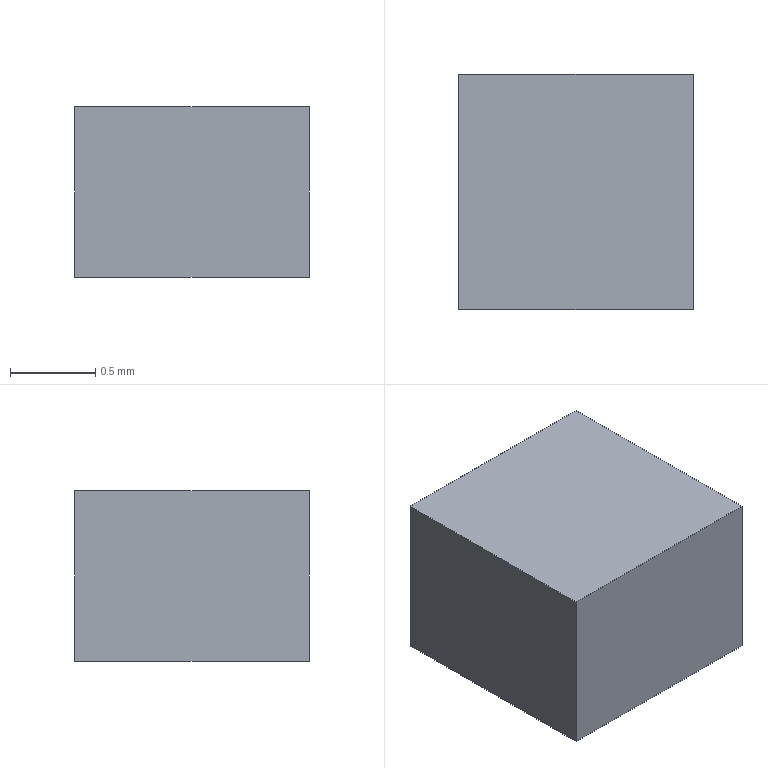Part | SolidWorks | features BaseBody 1 | 1 solid | 6 faces | box 1.375 x 1.375 x 1 mm | volume 1.891 mm3 | plane 6
STEP:
#1=CARTESIAN_POINT('',(7.625,9.125,1.5));
#2=VERTEX_POINT('',#1);
#3=CARTESIAN_POINT('',(7.625,7.75,1.5));
#4=VERTEX_POINT('',#3);
#5=CARTESIAN_POINT('',(7.625,9.125,1.5));
#6=DIRECTION('',(0.,-1.,0.));
#7=VECTOR('',#6,1000.);
#8=LINE('',#5,#7);
#9=EDGE_CURVE('',#2,#4,#8,.T.);
#10=ORIENTED_EDGE('',*,*,#9,.T.);
#11=CARTESIAN_POINT('',(7.625,7.75,2.5));
#12=VERTEX_POINT('',#11);
#13=CARTESIAN_POINT('',(7.625,7.75,2.5));
#14=DIRECTION('',(0.,0.,-1.));
#15=VECTOR('',#14,1000.);
#16=LINE('',#13,#15);
#17=EDGE_CURVE('',#12,#4,#16,.T.);
#18=ORIENTED_EDGE('',*,*,#17,.F.);
#19=CARTESIAN_POINT('',(7.625,9.125,2.5));
#20=VERTEX_POINT('',#19);
#21=CARTESIAN_POINT('',(7.625,9.125,2.5));
#22=DIRECTION('',(0.,-1.,0.));
#23=VECTOR('',#22,1000.);
#24=LINE('',#21,#23);
#25=EDGE_CURVE('',#20,#12,#24,.T.);
#26=ORIENTED_EDGE('',*,*,#25,.F.);
#27=CARTESIAN_POINT('',(7.625,9.125,2.5));
#28=DIRECTION('',(0.,0.,-1.));
#29=VECTOR('',#28,1000.);
#30=LINE('',#27,#29);
#31=EDGE_CURVE('',#20,#2,#30,.T.);
#32=ORIENTED_EDGE('',*,*,#31,.T.);
#33=EDGE_LOOP('',(#10,#18,#26,#32));
#34=FACE_OUTER_BOUND('',#33,.T.);
#35=CARTESIAN_POINT('',(7.625,9.125,2.5));
#36=DIRECTION('',(1.,0.,0.));
#37=DIRECTION('',(0.,0.,-1.));
#38=AXIS2_PLACEMENT_3D('',#35,#36,#37);
#39=PLANE('',#38);
#40=ADVANCED_FACE('',(#34),#39,.F.);
#41=CARTESIAN_POINT('',(9.,7.75,1.5));
#42=VERTEX_POINT('',#41);
#43=CARTESIAN_POINT('',(7.625,7.75,1.5));
#44=DIRECTION('',(1.,0.,0.));
#45=VECTOR('',#44,1000.);
#46=LINE('',#43,#45);
#47=EDGE_CURVE('',#4,#42,#46,.T.);
#48=ORIENTED_EDGE('',*,*,#47,.T.);
#49=CARTESIAN_POINT('',(9.,7.75,2.5));
#50=VERTEX_POINT('',#49);
#51=CARTESIAN_POINT('',(9.,7.75,2.5));
#52=DIRECTION('',(0.,0.,-1.));
#53=VECTOR('',#52,1000.);
#54=LINE('',#51,#53);
#55=EDGE_CURVE('',#50,#42,#54,.T.);
#56=ORIENTED_EDGE('',*,*,#55,.F.);
#57=CARTESIAN_POINT('',(7.625,7.75,2.5));
#58=DIRECTION('',(1.,0.,0.));
#59=VECTOR('',#58,1000.);
#60=LINE('',#57,#59);
#61=EDGE_CURVE('',#12,#50,#60,.T.);
#62=ORIENTED_EDGE('',*,*,#61,.F.);
#63=ORIENTED_EDGE('',*,*,#17,.T.);
#64=EDGE_LOOP('',(#48,#56,#62,#63));
#65=FACE_OUTER_BOUND('',#64,.T.);
#66=CARTESIAN_POINT('',(7.625,7.75,2.5));
#67=DIRECTION('',(0.,1.,0.));
#68=DIRECTION('',(0.,0.,1.));
#69=AXIS2_PLACEMENT_3D('',#66,#67,#68);
#70=PLANE('',#69);
#71=ADVANCED_FACE('',(#65),#70,.F.);
#72=CARTESIAN_POINT('',(9.,9.125,1.5));
#73=VERTEX_POINT('',#72);
#74=CARTESIAN_POINT('',(9.,7.75,1.5));
#75=DIRECTION('',(0.,1.,0.));
#76=VECTOR('',#75,1000.);
#77=LINE('',#74,#76);
#78=EDGE_CURVE('',#42,#73,#77,.T.);
#79=ORIENTED_EDGE('',*,*,#78,.T.);
#80=CARTESIAN_POINT('',(9.,9.125,2.5));
#81=VERTEX_POINT('',#80);
#82=CARTESIAN_POINT('',(9.,9.125,2.5));
#83=DIRECTION('',(0.,0.,-1.));
#84=VECTOR('',#83,1000.);
#85=LINE('',#82,#84);
#86=EDGE_CURVE('',#81,#73,#85,.T.);
#87=ORIENTED_EDGE('',*,*,#86,.F.);
#88=CARTESIAN_POINT('',(9.,7.75,2.5));
#89=DIRECTION('',(0.,1.,0.));
#90=VECTOR('',#89,1000.);
#91=LINE('',#88,#90);
#92=EDGE_CURVE('',#50,#81,#91,.T.);
#93=ORIENTED_EDGE('',*,*,#92,.F.);
#94=ORIENTED_EDGE('',*,*,#55,.T.);
#95=EDGE_LOOP('',(#79,#87,#93,#94));
#96=FACE_OUTER_BOUND('',#95,.T.);
#97=CARTESIAN_POINT('',(9.,7.75,2.5));
#98=DIRECTION('',(-1.,0.,0.));
#99=DIRECTION('',(0.,0.,1.));
#100=AXIS2_PLACEMENT_3D('',#97,#98,#99);
#101=PLANE('',#100);
#102=ADVANCED_FACE('',(#96),#101,.F.);
#103=CARTESIAN_POINT('',(9.,9.125,1.5));
#104=DIRECTION('',(-1.,0.,0.));
#105=VECTOR('',#104,1000.);
#106=LINE('',#103,#105);
#107=EDGE_CURVE('',#73,#2,#106,.T.);
#108=ORIENTED_EDGE('',*,*,#107,.T.);
#109=ORIENTED_EDGE('',*,*,#31,.F.);
#110=CARTESIAN_POINT('',(9.,9.125,2.5));
#111=DIRECTION('',(-1.,0.,0.));
#112=VECTOR('',#111,1000.);
#113=LINE('',#110,#112);
#114=EDGE_CURVE('',#81,#20,#113,.T.);
#115=ORIENTED_EDGE('',*,*,#114,.F.);
#116=ORIENTED_EDGE('',*,*,#86,.T.);
#117=EDGE_LOOP('',(#108,#109,#115,#116));
#118=FACE_OUTER_BOUND('',#117,.T.);
#119=CARTESIAN_POINT('',(9.,9.125,2.5));
#120=DIRECTION('',(0.,-1.,0.));
#121=DIRECTION('',(0.,0.,-1.));
#122=AXIS2_PLACEMENT_3D('',#119,#120,#121);
#123=PLANE('',#122);
#124=ADVANCED_FACE('',(#118),#123,.F.);
#125=ORIENTED_EDGE('',*,*,#25,.T.);
#126=ORIENTED_EDGE('',*,*,#61,.T.);
#127=ORIENTED_EDGE('',*,*,#92,.T.);
#128=ORIENTED_EDGE('',*,*,#114,.T.);
#129=EDGE_LOOP('',(#125,#126,#127,#128));
#130=FACE_OUTER_BOUND('',#129,.T.);
#131=CARTESIAN_POINT('',(0.,0.,2.5));
#132=DIRECTION('',(0.,0.,1.));
#133=DIRECTION('',(1.,0.,0.));
#134=AXIS2_PLACEMENT_3D('',#131,#132,#133);
#135=PLANE('',#134);
#136=ADVANCED_FACE('',(#130),#135,.T.);
#137=ORIENTED_EDGE('',*,*,#9,.F.);
#138=ORIENTED_EDGE('',*,*,#107,.F.);
#139=ORIENTED_EDGE('',*,*,#78,.F.);
#140=ORIENTED_EDGE('',*,*,#47,.F.);
#141=EDGE_LOOP('',(#137,#138,#139,#140));
#142=FACE_OUTER_BOUND('',#141,.T.);
#143=CARTESIAN_POINT('',(0.,0.,1.5));
#144=DIRECTION('',(0.,0.,1.));
#145=DIRECTION('',(1.,0.,0.));
#146=AXIS2_PLACEMENT_3D('',#143,#144,#145);
#147=PLANE('',#146);
#148=ADVANCED_FACE('',(#142),#147,.F.);
#149=CLOSED_SHELL('',(#40,#71,#102,#124,#136,#148));
#150=MANIFOLD_SOLID_BREP('',#149);
#151=CARTESIAN_POINT('',(0.,0.,0.));
#152=DIRECTION('',(0.,0.,1.));
#153=DIRECTION('',(1.,0.,0.));
#154=AXIS2_PLACEMENT_3D('',#151,#152,#153);
#155=(LENGTH_UNIT()NAMED_UNIT(*)SI_UNIT(.MILLI.,.METRE.));
#156=UNCERTAINTY_MEASURE_WITH_UNIT(LENGTH_MEASURE(0.00001),#155,'','');
#157=(NAMED_UNIT(*)PLANE_ANGLE_UNIT()SI_UNIT($,.RADIAN.));
#158=(NAMED_UNIT(*)SI_UNIT($,.STERADIAN.)SOLID_ANGLE_UNIT());
#159=(GEOMETRIC_REPRESENTATION_CONTEXT(3)GLOBAL_UNCERTAINTY_ASSIGNED_CONTEXT((#156))GLOBAL_UNIT_ASSIGNED_CONTEXT((#155,#157,#158))REPRESENTATION_CONTEXT('',''));
#160=ADVANCED_BREP_SHAPE_REPRESENTATION('',(#150,#154),#159);